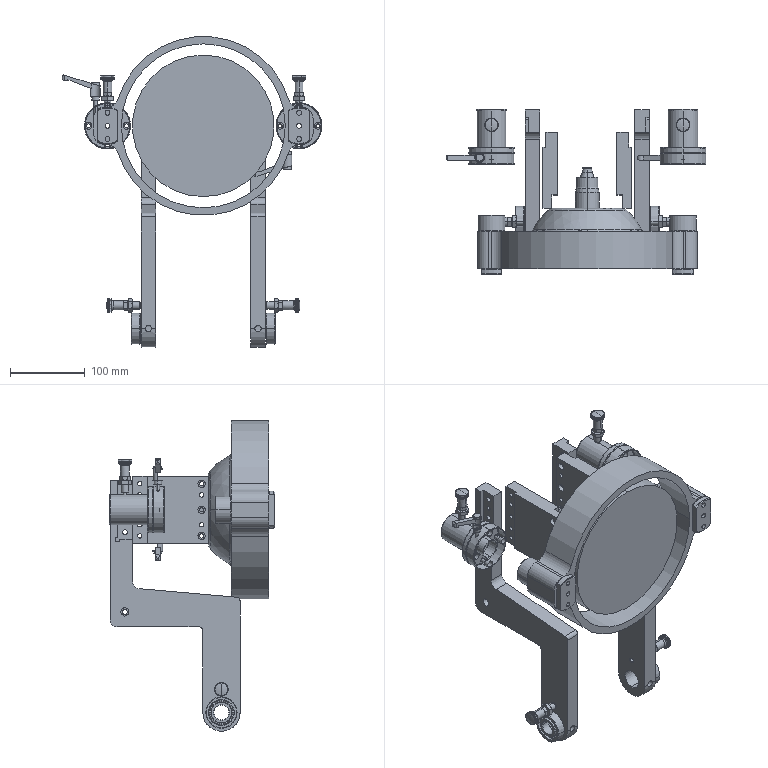Part | NX | features BREP 16 | 23 solids | 3544 faces | volume 3416190 mm3 | cylinder 1982 | plane 982 | torus 226 | cone 216 | sphere 138 | commonest cylinder face diameters 0.1 x896 17.4 x360 18 x360 10 x36 5.5 x32 6.5 x32